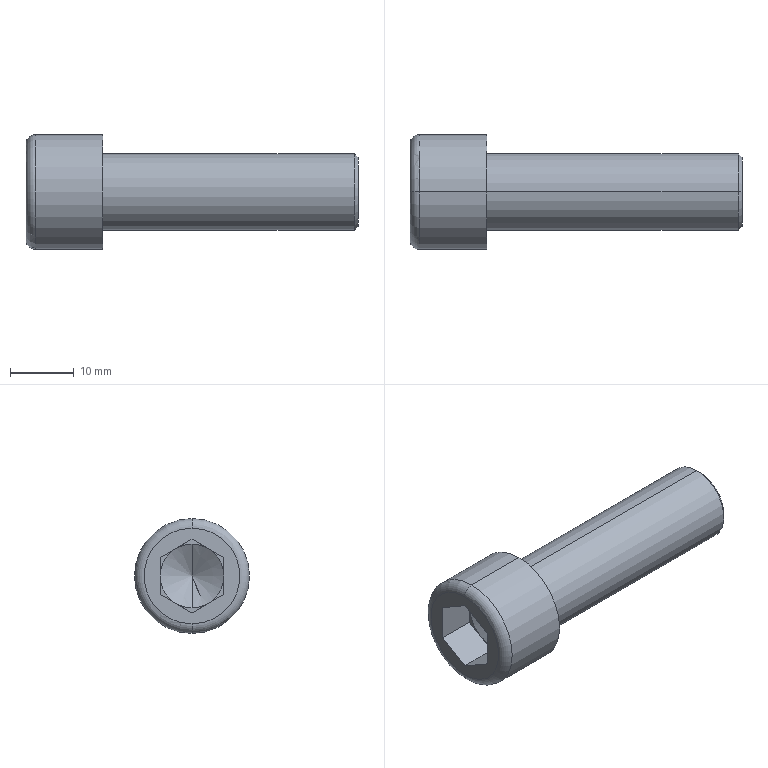Part | SolidWorks | features BaseBody 1 | 1 solid | 25 faces | box 52 x 18 x 18 mm | volume 6949 mm3 | plane 15 | cone 4 | cylinder 4 | torus 2 | commonest cylinder face diameters 12 x2 18 x2
STEP:
#1=CARTESIAN_POINT('',(52.,0.,-5.4));
#2=VERTEX_POINT('',#1);
#3=CARTESIAN_POINT('',(52.,0.,5.4));
#4=VERTEX_POINT('',#3);
#5=CARTESIAN_POINT('',(52.,0.,0.));
#6=DIRECTION('',(1.,0.,0.));
#7=DIRECTION('',(0.,0.,-1.));
#8=AXIS2_PLACEMENT_3D('',#5,#6,#7);
#9=CIRCLE('',#8,5.4);
#10=EDGE_CURVE('',#2,#4,#9,.T.);
#11=ORIENTED_EDGE('',*,*,#10,.F.);
#12=CARTESIAN_POINT('',(51.4,0.,-6.));
#13=VERTEX_POINT('',#12);
#14=CARTESIAN_POINT('',(52.,0.,-5.4));
#15=DIRECTION('',(-0.7071,0.,-0.7071));
#16=VECTOR('',#15,1000.);
#17=LINE('',#14,#16);
#18=EDGE_CURVE('',#2,#13,#17,.T.);
#19=ORIENTED_EDGE('',*,*,#18,.T.);
#20=CARTESIAN_POINT('',(51.4,0.,6.));
#21=VERTEX_POINT('',#20);
#22=CARTESIAN_POINT('',(51.4,0.,0.));
#23=DIRECTION('',(-1.,0.,0.));
#24=DIRECTION('',(0.,0.,-1.));
#25=AXIS2_PLACEMENT_3D('',#22,#23,#24);
#26=CIRCLE('',#25,6.);
#27=EDGE_CURVE('',#21,#13,#26,.T.);
#28=ORIENTED_EDGE('',*,*,#27,.F.);
#29=CARTESIAN_POINT('',(52.,0.,5.4));
#30=DIRECTION('',(-0.7071,0.,0.7071));
#31=VECTOR('',#30,1000.);
#32=LINE('',#29,#31);
#33=EDGE_CURVE('',#4,#21,#32,.T.);
#34=ORIENTED_EDGE('',*,*,#33,.F.);
#35=EDGE_LOOP('',(#11,#19,#28,#34));
#36=FACE_OUTER_BOUND('',#35,.T.);
#37=CARTESIAN_POINT('',(52.,0.,0.));
#38=DIRECTION('',(-1.,0.,0.));
#39=DIRECTION('',(0.,0.,1.));
#40=AXIS2_PLACEMENT_3D('',#37,#38,#39);
#41=CONICAL_SURFACE('',#40,5.4,0.7854);
#42=ADVANCED_FACE('',(#36),#41,.T.);
#43=CARTESIAN_POINT('',(0.,0.,7.5));
#44=VERTEX_POINT('',#43);
#45=CARTESIAN_POINT('',(0.,0.,-7.5));
#46=VERTEX_POINT('',#45);
#47=CARTESIAN_POINT('',(0.,0.,0.));
#48=DIRECTION('',(-1.,0.,0.));
#49=DIRECTION('',(0.,0.,-1.));
#50=AXIS2_PLACEMENT_3D('',#47,#48,#49);
#51=CIRCLE('',#50,7.5);
#52=EDGE_CURVE('',#44,#46,#51,.T.);
#53=ORIENTED_EDGE('',*,*,#52,.F.);
#54=CARTESIAN_POINT('',(1.5,0.,9.));
#55=VERTEX_POINT('',#54);
#56=CARTESIAN_POINT('',(1.5,0.,7.5));
#57=DIRECTION('',(0.,1.,0.));
#58=DIRECTION('',(0.,0.,1.));
#59=AXIS2_PLACEMENT_3D('',#56,#57,#58);
#60=CIRCLE('',#59,1.5);
#61=EDGE_CURVE('',#44,#55,#60,.T.);
#62=ORIENTED_EDGE('',*,*,#61,.T.);
#63=CARTESIAN_POINT('',(1.5,0.,-9.));
#64=VERTEX_POINT('',#63);
#65=CARTESIAN_POINT('',(1.5,0.,0.));
#66=DIRECTION('',(1.,0.,0.));
#67=DIRECTION('',(0.,0.,-1.));
#68=AXIS2_PLACEMENT_3D('',#65,#66,#67);
#69=CIRCLE('',#68,9.);
#70=EDGE_CURVE('',#64,#55,#69,.T.);
#71=ORIENTED_EDGE('',*,*,#70,.F.);
#72=CARTESIAN_POINT('',(1.5,0.,-7.5));
#73=DIRECTION('',(0.,-1.,0.));
#74=DIRECTION('',(0.,0.,-1.));
#75=AXIS2_PLACEMENT_3D('',#72,#73,#74);
#76=CIRCLE('',#75,1.5);
#77=EDGE_CURVE('',#46,#64,#76,.T.);
#78=ORIENTED_EDGE('',*,*,#77,.F.);
#79=EDGE_LOOP('',(#53,#62,#71,#78));
#80=FACE_OUTER_BOUND('',#79,.T.);
#81=CARTESIAN_POINT('',(1.5,0.,0.));
#82=DIRECTION('',(1.,0.,0.));
#83=DIRECTION('',(0.,0.,-1.));
#84=AXIS2_PLACEMENT_3D('',#81,#82,#83);
#85=TOROIDAL_SURFACE('',#84,7.5,1.5);
#86=ADVANCED_FACE('',(#80),#85,.T.);
#87=CARTESIAN_POINT('',(8.887,0.,0.));
#88=VERTEX_POINT('',#87);
#89=CARTESIAN_POINT('',(6.,0.,5.));
#90=VERTEX_POINT('',#89);
#91=CARTESIAN_POINT('',(6.,0.,5.));
#92=DIRECTION('',(-0.5,0.,0.866));
#93=VECTOR('',#92,1000.);
#94=LINE('',#91,#93);
#95=EDGE_CURVE('',#88,#90,#94,.T.);
#96=ORIENTED_EDGE('',*,*,#95,.F.);
#97=CARTESIAN_POINT('',(6.,0.,-5.));
#98=VERTEX_POINT('',#97);
#99=CARTESIAN_POINT('',(6.,0.,-5.));
#100=DIRECTION('',(-0.5,0.,-0.866));
#101=VECTOR('',#100,1000.);
#102=LINE('',#99,#101);
#103=EDGE_CURVE('',#88,#98,#102,.T.);
#104=ORIENTED_EDGE('',*,*,#103,.T.);
#105=CARTESIAN_POINT('',(6.,-2.5,-4.33));
#106=VERTEX_POINT('',#105);
#107=CARTESIAN_POINT('',(6.,0.,0.));
#108=DIRECTION('',(-1.,0.,0.));
#109=DIRECTION('',(0.,0.,-1.));
#110=AXIS2_PLACEMENT_3D('',#107,#108,#109);
#111=CIRCLE('',#110,5.);
#112=EDGE_CURVE('',#98,#106,#111,.T.);
#113=ORIENTED_EDGE('',*,*,#112,.T.);
#114=CARTESIAN_POINT('',(6.,-5.,0.));
#115=VERTEX_POINT('',#114);
#116=CARTESIAN_POINT('',(6.,0.,0.));
#117=DIRECTION('',(-1.,0.,0.));
#118=DIRECTION('',(0.,0.,-1.));
#119=AXIS2_PLACEMENT_3D('',#116,#117,#118);
#120=CIRCLE('',#119,5.);
#121=EDGE_CURVE('',#106,#115,#120,.T.);
#122=ORIENTED_EDGE('',*,*,#121,.T.);
#123=CARTESIAN_POINT('',(6.,-2.5,4.33));
#124=VERTEX_POINT('',#123);
#125=CARTESIAN_POINT('',(6.,0.,0.));
#126=DIRECTION('',(-1.,0.,0.));
#127=DIRECTION('',(0.,0.,-1.));
#128=AXIS2_PLACEMENT_3D('',#125,#126,#127);
#129=CIRCLE('',#128,5.);
#130=EDGE_CURVE('',#115,#124,#129,.T.);
#131=ORIENTED_EDGE('',*,*,#130,.T.);
#132=CARTESIAN_POINT('',(6.,0.,0.));
#133=DIRECTION('',(-1.,0.,0.));
#134=DIRECTION('',(0.,0.,-1.));
#135=AXIS2_PLACEMENT_3D('',#132,#133,#134);
#136=CIRCLE('',#135,5.);
#137=EDGE_CURVE('',#124,#90,#136,.T.);
#138=ORIENTED_EDGE('',*,*,#137,.T.);
#139=EDGE_LOOP('',(#96,#104,#113,#122,#131,#138));
#140=FACE_OUTER_BOUND('',#139,.T.);
#141=CARTESIAN_POINT('',(6.,0.,0.));
#142=DIRECTION('',(-1.,0.,0.));
#143=DIRECTION('',(0.,0.,1.));
#144=AXIS2_PLACEMENT_3D('',#141,#142,#143);
#145=CONICAL_SURFACE('',#144,5.,1.047);
#146=ADVANCED_FACE('',(#140),#145,.F.);
#147=ORIENTED_EDGE('',*,*,#27,.T.);
#148=CARTESIAN_POINT('',(12.,0.,-6.));
#149=VERTEX_POINT('',#148);
#150=CARTESIAN_POINT('',(52.,0.,-6.));
#151=DIRECTION('',(-1.,0.,0.));
#152=VECTOR('',#151,1000.);
#153=LINE('',#150,#152);
#154=EDGE_CURVE('',#13,#149,#153,.T.);
#155=ORIENTED_EDGE('',*,*,#154,.T.);
#156=CARTESIAN_POINT('',(12.,0.,6.));
#157=VERTEX_POINT('',#156);
#158=CARTESIAN_POINT('',(12.,0.,0.));
#159=DIRECTION('',(1.,0.,0.));
#160=DIRECTION('',(0.,0.,-1.));
#161=AXIS2_PLACEMENT_3D('',#158,#159,#160);
#162=CIRCLE('',#161,6.);
#163=EDGE_CURVE('',#149,#157,#162,.T.);
#164=ORIENTED_EDGE('',*,*,#163,.T.);
#165=CARTESIAN_POINT('',(52.,0.,6.));
#166=DIRECTION('',(-1.,0.,0.));
#167=VECTOR('',#166,1000.);
#168=LINE('',#165,#167);
#169=EDGE_CURVE('',#21,#157,#168,.T.);
#170=ORIENTED_EDGE('',*,*,#169,.F.);
#171=EDGE_LOOP('',(#147,#155,#164,#170));
#172=FACE_OUTER_BOUND('',#171,.T.);
#173=CARTESIAN_POINT('',(52.,0.,0.));
#174=DIRECTION('',(-1.,0.,0.));
#175=DIRECTION('',(0.,0.,1.));
#176=AXIS2_PLACEMENT_3D('',#173,#174,#175);
#177=CYLINDRICAL_SURFACE('',#176,6.);
#178=ADVANCED_FACE('',(#172),#177,.T.);
#179=CARTESIAN_POINT('',(12.,0.,-9.));
#180=VERTEX_POINT('',#179);
#181=CARTESIAN_POINT('',(12.,0.,9.));
#182=VERTEX_POINT('',#181);
#183=CARTESIAN_POINT('',(12.,0.,0.));
#184=DIRECTION('',(1.,0.,0.));
#185=DIRECTION('',(0.,0.,-1.));
#186=AXIS2_PLACEMENT_3D('',#183,#184,#185);
#187=CIRCLE('',#186,9.);
#188=EDGE_CURVE('',#180,#182,#187,.T.);
#189=ORIENTED_EDGE('',*,*,#188,.F.);
#190=CARTESIAN_POINT('',(12.,0.,-9.));
#191=DIRECTION('',(-1.,0.,0.));
#192=VECTOR('',#191,1000.);
#193=LINE('',#190,#192);
#194=EDGE_CURVE('',#180,#64,#193,.T.);
#195=ORIENTED_EDGE('',*,*,#194,.T.);
#196=ORIENTED_EDGE('',*,*,#70,.T.);
#197=CARTESIAN_POINT('',(12.,0.,9.));
#198=DIRECTION('',(-1.,0.,0.));
#199=VECTOR('',#198,1000.);
#200=LINE('',#197,#199);
#201=EDGE_CURVE('',#182,#55,#200,.T.);
#202=ORIENTED_EDGE('',*,*,#201,.F.);
#203=EDGE_LOOP('',(#189,#195,#196,#202));
#204=FACE_OUTER_BOUND('',#203,.T.);
#205=CARTESIAN_POINT('',(12.,0.,0.));
#206=DIRECTION('',(-1.,0.,0.));
#207=DIRECTION('',(0.,0.,1.));
#208=AXIS2_PLACEMENT_3D('',#205,#206,#207);
#209=CYLINDRICAL_SURFACE('',#208,9.);
#210=ADVANCED_FACE('',(#204),#209,.T.);
#211=CARTESIAN_POINT('',(0.,-5.,2.887));
#212=VERTEX_POINT('',#211);
#213=CARTESIAN_POINT('',(0.,-5.,-2.887));
#214=VERTEX_POINT('',#213);
#215=CARTESIAN_POINT('',(0.,-5.,2.887));
#216=DIRECTION('',(0.,0.,-1.));
#217=VECTOR('',#216,1000.);
#218=LINE('',#215,#217);
#219=EDGE_CURVE('',#212,#214,#218,.T.);
#220=ORIENTED_EDGE('',*,*,#219,.F.);
#221=CARTESIAN_POINT('',(6.,-5.,2.887));
#222=VERTEX_POINT('',#221);
#223=CARTESIAN_POINT('',(6.,-5.,2.887));
#224=DIRECTION('',(-1.,0.,0.));
#225=VECTOR('',#224,1000.);
#226=LINE('',#223,#225);
#227=EDGE_CURVE('',#222,#212,#226,.T.);
#228=ORIENTED_EDGE('',*,*,#227,.F.);
#229=CARTESIAN_POINT('',(6.,-5.,2.887));
#230=DIRECTION('',(0.,0.,-1.));
#231=VECTOR('',#230,1000.);
#232=LINE('',#229,#231);
#233=EDGE_CURVE('',#222,#115,#232,.T.);
#234=ORIENTED_EDGE('',*,*,#233,.T.);
#235=CARTESIAN_POINT('',(6.,-5.,-2.887));
#236=VERTEX_POINT('',#235);
#237=CARTESIAN_POINT('',(6.,-5.,2.887));
#238=DIRECTION('',(0.,0.,-1.));
#239=VECTOR('',#238,1000.);
#240=LINE('',#237,#239);
#241=EDGE_CURVE('',#115,#236,#240,.T.);
#242=ORIENTED_EDGE('',*,*,#241,.T.);
#243=CARTESIAN_POINT('',(6.,-5.,-2.887));
#244=DIRECTION('',(-1.,0.,0.));
#245=VECTOR('',#244,1000.);
#246=LINE('',#243,#245);
#247=EDGE_CURVE('',#236,#214,#246,.T.);
#248=ORIENTED_EDGE('',*,*,#247,.T.);
#249=EDGE_LOOP('',(#220,#228,#234,#242,#248));
#250=FACE_OUTER_BOUND('',#249,.T.);
#251=CARTESIAN_POINT('',(6.,-5.,2.887));
#252=DIRECTION('',(0.,1.,0.));
#253=DIRECTION('',(1.,0.,0.));
#254=AXIS2_PLACEMENT_3D('',#251,#252,#253);
#255=PLANE('',#254);
#256=ADVANCED_FACE('',(#250),#255,.T.);
#257=CARTESIAN_POINT('',(0.,0.,5.774));
#258=VERTEX_POINT('',#257);
#259=CARTESIAN_POINT('',(0.,0.,5.774));
#260=DIRECTION('',(0.,-0.866,-0.5));
#261=VECTOR('',#260,1000.);
#262=LINE('',#259,#261);
#263=EDGE_CURVE('',#258,#212,#262,.T.);
#264=ORIENTED_EDGE('',*,*,#263,.F.);
#265=CARTESIAN_POINT('',(6.,0.,5.774));
#266=VERTEX_POINT('',#265);
#267=CARTESIAN_POINT('',(6.,0.,5.774));
#268=DIRECTION('',(-1.,0.,0.));
#269=VECTOR('',#268,1000.);
#270=LINE('',#267,#269);
#271=EDGE_CURVE('',#266,#258,#270,.T.);
#272=ORIENTED_EDGE('',*,*,#271,.F.);
#273=CARTESIAN_POINT('',(6.,0.,5.774));
#274=DIRECTION('',(0.,-0.866,-0.5));
#275=VECTOR('',#274,1000.);
#276=LINE('',#273,#275);
#277=EDGE_CURVE('',#266,#124,#276,.T.);
#278=ORIENTED_EDGE('',*,*,#277,.T.);
#279=CARTESIAN_POINT('',(6.,0.,5.774));
#280=DIRECTION('',(0.,-0.866,-0.5));
#281=VECTOR('',#280,1000.);
#282=LINE('',#279,#281);
#283=EDGE_CURVE('',#124,#222,#282,.T.);
#284=ORIENTED_EDGE('',*,*,#283,.T.);
#285=ORIENTED_EDGE('',*,*,#227,.T.);
#286=EDGE_LOOP('',(#264,#272,#278,#284,#285));
#287=FACE_OUTER_BOUND('',#286,.T.);
#288=CARTESIAN_POINT('',(6.,0.,5.774));
#289=DIRECTION('',(0.,0.5,-0.866));
#290=DIRECTION('',(-1.,0.,0.));
#291=AXIS2_PLACEMENT_3D('',#288,#289,#290);
#292=PLANE('',#291);
#293=ADVANCED_FACE('',(#287),#292,.T.);
#294=CARTESIAN_POINT('',(0.,5.,2.887));
#295=VERTEX_POINT('',#294);
#296=CARTESIAN_POINT('',(0.,5.,2.887));
#297=DIRECTION('',(0.,-0.866,0.5));
#298=VECTOR('',#297,1000.);
#299=LINE('',#296,#298);
#300=EDGE_CURVE('',#295,#258,#299,.T.);
#301=ORIENTED_EDGE('',*,*,#300,.F.);
#302=CARTESIAN_POINT('',(6.,5.,2.887));
#303=VERTEX_POINT('',#302);
#304=CARTESIAN_POINT('',(6.,5.,2.887));
#305=DIRECTION('',(-1.,0.,0.));
#306=VECTOR('',#305,1000.);
#307=LINE('',#304,#306);
#308=EDGE_CURVE('',#303,#295,#307,.T.);
#309=ORIENTED_EDGE('',*,*,#308,.F.);
#310=CARTESIAN_POINT('',(6.,2.5,4.33));
#311=VERTEX_POINT('',#310);
#312=CARTESIAN_POINT('',(6.,5.,2.887));
#313=DIRECTION('',(0.,-0.866,0.5));
#314=VECTOR('',#313,1000.);
#315=LINE('',#312,#314);
#316=EDGE_CURVE('',#303,#311,#315,.T.);
#317=ORIENTED_EDGE('',*,*,#316,.T.);
#318=CARTESIAN_POINT('',(6.,5.,2.887));
#319=DIRECTION('',(0.,-0.866,0.5));
#320=VECTOR('',#319,1000.);
#321=LINE('',#318,#320);
#322=EDGE_CURVE('',#311,#266,#321,.T.);
#323=ORIENTED_EDGE('',*,*,#322,.T.);
#324=ORIENTED_EDGE('',*,*,#271,.T.);
#325=EDGE_LOOP('',(#301,#309,#317,#323,#324));
#326=FACE_OUTER_BOUND('',#325,.T.);
#327=CARTESIAN_POINT('',(6.,5.,2.887));
#328=DIRECTION('',(0.,-0.5,-0.866));
#329=DIRECTION('',(0.,-0.866,0.5));
#330=AXIS2_PLACEMENT_3D('',#327,#328,#329);
#331=PLANE('',#330);
#332=ADVANCED_FACE('',(#326),#331,.T.);
#333=CARTESIAN_POINT('',(0.,5.,-2.887));
#334=VERTEX_POINT('',#333);
#335=CARTESIAN_POINT('',(0.,5.,-2.887));
#336=DIRECTION('',(0.,0.,1.));
#337=VECTOR('',#336,1000.);
#338=LINE('',#335,#337);
#339=EDGE_CURVE('',#334,#295,#338,.T.);
#340=ORIENTED_EDGE('',*,*,#339,.F.);
#341=CARTESIAN_POINT('',(6.,5.,-2.887));
#342=VERTEX_POINT('',#341);
#343=CARTESIAN_POINT('',(6.,5.,-2.887));
#344=DIRECTION('',(-1.,0.,0.));
#345=VECTOR('',#344,1000.);
#346=LINE('',#343,#345);
#347=EDGE_CURVE('',#342,#334,#346,.T.);
#348=ORIENTED_EDGE('',*,*,#347,.F.);
#349=CARTESIAN_POINT('',(6.,5.,0.));
#350=VERTEX_POINT('',#349);
#351=CARTESIAN_POINT('',(6.,5.,-2.887));
#352=DIRECTION('',(0.,0.,1.));
#353=VECTOR('',#352,1000.);
#354=LINE('',#351,#353);
#355=EDGE_CURVE('',#342,#350,#354,.T.);
#356=ORIENTED_EDGE('',*,*,#355,.T.);
#357=CARTESIAN_POINT('',(6.,5.,-2.887));
#358=DIRECTION('',(0.,0.,1.));
#359=VECTOR('',#358,1000.);
#360=LINE('',#357,#359);
#361=EDGE_CURVE('',#350,#303,#360,.T.);
#362=ORIENTED_EDGE('',*,*,#361,.T.);
#363=ORIENTED_EDGE('',*,*,#308,.T.);
#364=EDGE_LOOP('',(#340,#348,#356,#362,#363));
#365=FACE_OUTER_BOUND('',#364,.T.);
#366=CARTESIAN_POINT('',(6.,5.,-2.887));
#367=DIRECTION('',(0.,-1.,0.));
#368=DIRECTION('',(0.,0.,-1.));
#369=AXIS2_PLACEMENT_3D('',#366,#367,#368);
#370=PLANE('',#369);
#371=ADVANCED_FACE('',(#365),#370,.T.);
#372=CARTESIAN_POINT('',(0.,0.,-5.774));
#373=VERTEX_POINT('',#372);
#374=CARTESIAN_POINT('',(0.,0.,-5.774));
#375=DIRECTION('',(0.,0.866,0.5));
#376=VECTOR('',#375,1000.);
#377=LINE('',#374,#376);
#378=EDGE_CURVE('',#373,#334,#377,.T.);
#379=ORIENTED_EDGE('',*,*,#378,.F.);
#380=CARTESIAN_POINT('',(6.,0.,-5.774));
#381=VERTEX_POINT('',#380);
#382=CARTESIAN_POINT('',(6.,0.,-5.774));
#383=DIRECTION('',(-1.,0.,0.));
#384=VECTOR('',#383,1000.);
#385=LINE('',#382,#384);
#386=EDGE_CURVE('',#381,#373,#385,.T.);
#387=ORIENTED_EDGE('',*,*,#386,.F.);
#388=CARTESIAN_POINT('',(6.,2.5,-4.33));
#389=VERTEX_POINT('',#388);
#390=CARTESIAN_POINT('',(6.,0.,-5.774));
#391=DIRECTION('',(0.,0.866,0.5));
#392=VECTOR('',#391,1000.);
#393=LINE('',#390,#392);
#394=EDGE_CURVE('',#381,#389,#393,.T.);
#395=ORIENTED_EDGE('',*,*,#394,.T.);
#396=CARTESIAN_POINT('',(6.,0.,-5.774));
#397=DIRECTION('',(0.,0.866,0.5));
#398=VECTOR('',#397,1000.);
#399=LINE('',#396,#398);
#400=EDGE_CURVE('',#389,#342,#399,.T.);
#401=ORIENTED_EDGE('',*,*,#400,.T.);
#402=ORIENTED_EDGE('',*,*,#347,.T.);
#403=EDGE_LOOP('',(#379,#387,#395,#401,#402));
#404=FACE_OUTER_BOUND('',#403,.T.);
#405=CARTESIAN_POINT('',(6.,0.,-5.774));
#406=DIRECTION('',(0.,-0.5,0.866));
#407=DIRECTION('',(-1.,0.,0.));
#408=AXIS2_PLACEMENT_3D('',#405,#406,#407);
#409=PLANE('',#408);
#410=ADVANCED_FACE('',(#404),#409,.T.);
#411=CARTESIAN_POINT('',(0.,-5.,-2.887));
#412=DIRECTION('',(0.,0.866,-0.5));
#413=VECTOR('',#412,1000.);
#414=LINE('',#411,#413);
#415=EDGE_CURVE('',#214,#373,#414,.T.);
#416=ORIENTED_EDGE('',*,*,#415,.F.);
#417=ORIENTED_EDGE('',*,*,#247,.F.);
#418=CARTESIAN_POINT('',(6.,-5.,-2.887));
#419=DIRECTION('',(0.,0.866,-0.5));
#420=VECTOR('',#419,1000.);
#421=LINE('',#418,#420);
#422=EDGE_CURVE('',#236,#106,#421,.T.);
#423=ORIENTED_EDGE('',*,*,#422,.T.);
#424=CARTESIAN_POINT('',(6.,-5.,-2.887));
#425=DIRECTION('',(0.,0.866,-0.5));
#426=VECTOR('',#425,1000.);
#427=LINE('',#424,#426);
#428=EDGE_CURVE('',#106,#381,#427,.T.);
#429=ORIENTED_EDGE('',*,*,#428,.T.);
#430=ORIENTED_EDGE('',*,*,#386,.T.);
#431=EDGE_LOOP('',(#416,#417,#423,#429,#430));
#432=FACE_OUTER_BOUND('',#431,.T.);
#433=CARTESIAN_POINT('',(6.,-5.,-2.887));
#434=DIRECTION('',(0.,0.5,0.866));
#435=DIRECTION('',(1.,0.,0.));
#436=AXIS2_PLACEMENT_3D('',#433,#434,#435);
#437=PLANE('',#436);
#438=ADVANCED_FACE('',(#432),#437,.T.);
#439=CARTESIAN_POINT('',(52.,0.,0.));
#440=DIRECTION('',(1.,0.,0.));
#441=DIRECTION('',(0.,0.,-1.));
#442=AXIS2_PLACEMENT_3D('',#439,#440,#441);
#443=CIRCLE('',#442,5.4);
#444=EDGE_CURVE('',#4,#2,#443,.T.);
#445=ORIENTED_EDGE('',*,*,#444,.T.);
#446=ORIENTED_EDGE('',*,*,#10,.T.);
#447=EDGE_LOOP('',(#445,#446));
#448=FACE_OUTER_BOUND('',#447,.T.);
#449=CARTESIAN_POINT('',(52.,0.,0.));
#450=DIRECTION('',(1.,0.,0.));
#451=DIRECTION('',(0.,1.,0.));
#452=AXIS2_PLACEMENT_3D('',#449,#450,#451);
#453=PLANE('',#452);
#454=ADVANCED_FACE('',(#448),#453,.T.);
#455=CARTESIAN_POINT('',(12.,0.,0.));
#456=DIRECTION('',(1.,0.,0.));
#457=DIRECTION('',(0.,0.,-1.));
#458=AXIS2_PLACEMENT_3D('',#455,#456,#457);
#459=CIRCLE('',#458,6.);
#460=EDGE_CURVE('',#157,#149,#459,.T.);
#461=ORIENTED_EDGE('',*,*,#460,.F.);
#462=ORIENTED_EDGE('',*,*,#163,.F.);
#463=EDGE_LOOP('',(#461,#462));
#464=FACE_BOUND('',#463,.T.);
#465=CARTESIAN_POINT('',(12.,0.,0.));
#466=DIRECTION('',(1.,0.,0.));
#467=DIRECTION('',(0.,0.,-1.));
#468=AXIS2_PLACEMENT_3D('',#465,#466,#467);
#469=CIRCLE('',#468,9.);
#470=EDGE_CURVE('',#182,#180,#469,.T.);
#471=ORIENTED_EDGE('',*,*,#470,.T.);
#472=ORIENTED_EDGE('',*,*,#188,.T.);
#473=EDGE_LOOP('',(#471,#472));
#474=FACE_OUTER_BOUND('',#473,.T.);
#475=CARTESIAN_POINT('',(12.,0.,0.));
#476=DIRECTION('',(1.,0.,0.));
#477=DIRECTION('',(0.,1.,0.));
#478=AXIS2_PLACEMENT_3D('',#475,#476,#477);
#479=PLANE('',#478);
#480=ADVANCED_FACE('',(#464,#474),#479,.T.);
#481=ORIENTED_EDGE('',*,*,#415,.T.);
#482=ORIENTED_EDGE('',*,*,#378,.T.);
#483=ORIENTED_EDGE('',*,*,#339,.T.);
#484=ORIENTED_EDGE('',*,*,#300,.T.);
#485=ORIENTED_EDGE('',*,*,#263,.T.);
#486=ORIENTED_EDGE('',*,*,#219,.T.);
#487=EDGE_LOOP('',(#481,#482,#483,#484,#485,#486));
#488=FACE_BOUND('',#487,.T.);
#489=CARTESIAN_POINT('',(0.,0.,0.));
#490=DIRECTION('',(-1.,0.,0.));
#491=DIRECTION('',(0.,0.,-1.));
#492=AXIS2_PLACEMENT_3D('',#489,#490,#491);
#493=CIRCLE('',#492,7.5);
#494=EDGE_CURVE('',#46,#44,#493,.T.);
#495=ORIENTED_EDGE('',*,*,#494,.T.);
#496=ORIENTED_EDGE('',*,*,#52,.T.);
#497=EDGE_LOOP('',(#495,#496));
#498=FACE_OUTER_BOUND('',#497,.T.);
#499=CARTESIAN_POINT('',(0.,0.,0.));
#500=DIRECTION('',(1.,0.,0.));
#501=DIRECTION('',(0.,1.,0.));
#502=AXIS2_PLACEMENT_3D('',#499,#500,#501);
#503=PLANE('',#502);
#504=ADVANCED_FACE('',(#488,#498),#503,.F.);
#505=CARTESIAN_POINT('',(6.,0.,0.));
#506=DIRECTION('',(-1.,0.,0.));
#507=DIRECTION('',(0.,0.,-1.));
#508=AXIS2_PLACEMENT_3D('',#505,#506,#507);
#509=CIRCLE('',#508,5.);
#510=EDGE_CURVE('',#389,#98,#509,.T.);
#511=ORIENTED_EDGE('',*,*,#510,.F.);
#512=ORIENTED_EDGE('',*,*,#394,.F.);
#513=ORIENTED_EDGE('',*,*,#428,.F.);
#514=ORIENTED_EDGE('',*,*,#112,.F.);
#515=EDGE_LOOP('',(#511,#512,#513,#514));
#516=FACE_OUTER_BOUND('',#515,.T.);
#517=CARTESIAN_POINT('',(6.,0.,-5.774));
#518=DIRECTION('',(1.,0.,0.));
#519=DIRECTION('',(0.,1.,0.));
#520=AXIS2_PLACEMENT_3D('',#517,#518,#519);
#521=PLANE('',#520);
#522=ADVANCED_FACE('',(#516),#521,.F.);
#523=CARTESIAN_POINT('',(6.,0.,0.));
#524=DIRECTION('',(1.,0.,0.));
#525=DIRECTION('',(0.,0.,-1.));
#526=AXIS2_PLACEMENT_3D('',#523,#524,#525);
#527=CIRCLE('',#526,5.);
#528=EDGE_CURVE('',#389,#350,#527,.T.);
#529=ORIENTED_EDGE('',*,*,#528,.T.);
#530=ORIENTED_EDGE('',*,*,#355,.F.);
#531=ORIENTED_EDGE('',*,*,#400,.F.);
#532=EDGE_LOOP('',(#529,#530,#531));
#533=FACE_OUTER_BOUND('',#532,.T.);
#534=CARTESIAN_POINT('',(6.,0.,-5.774));
#535=DIRECTION('',(1.,0.,0.));
#536=DIRECTION('',(0.,1.,0.));
#537=AXIS2_PLACEMENT_3D('',#534,#535,#536);
#538=PLANE('',#537);
#539=ADVANCED_FACE('',(#533),#538,.F.);
#540=CARTESIAN_POINT('',(6.,0.,0.));
#541=DIRECTION('',(-1.,0.,0.));
#542=DIRECTION('',(0.,0.,-1.));
#543=AXIS2_PLACEMENT_3D('',#540,#541,#542);
#544=CIRCLE('',#543,5.);
#545=EDGE_CURVE('',#311,#350,#544,.T.);
#546=ORIENTED_EDGE('',*,*,#545,.F.);
#547=ORIENTED_EDGE('',*,*,#316,.F.);
#548=ORIENTED_EDGE('',*,*,#361,.F.);
#549=EDGE_LOOP('',(#546,#547,#548));
#550=FACE_OUTER_BOUND('',#549,.T.);
#551=CARTESIAN_POINT('',(6.,0.,-5.774));
#552=DIRECTION('',(1.,0.,0.));
#553=DIRECTION('',(0.,1.,0.));
#554=AXIS2_PLACEMENT_3D('',#551,#552,#553);
#555=PLANE('',#554);
#556=ADVANCED_FACE('',(#550),#555,.F.);
#557=ORIENTED_EDGE('',*,*,#137,.F.);
#558=ORIENTED_EDGE('',*,*,#277,.F.);
#559=ORIENTED_EDGE('',*,*,#322,.F.);
#560=CARTESIAN_POINT('',(6.,0.,0.));
#561=DIRECTION('',(-1.,0.,0.));
#562=DIRECTION('',(0.,0.,-1.));
#563=AXIS2_PLACEMENT_3D('',#560,#561,#562);
#564=CIRCLE('',#563,5.);
#565=EDGE_CURVE('',#90,#311,#564,.T.);
#566=ORIENTED_EDGE('',*,*,#565,.F.);
#567=EDGE_LOOP('',(#557,#558,#559,#566));
#568=FACE_OUTER_BOUND('',#567,.T.);
#569=CARTESIAN_POINT('',(6.,0.,-5.774));
#570=DIRECTION('',(1.,0.,0.));
#571=DIRECTION('',(0.,1.,0.));
#572=AXIS2_PLACEMENT_3D('',#569,#570,#571);
#573=PLANE('',#572);
#574=ADVANCED_FACE('',(#568),#573,.F.);
#575=ORIENTED_EDGE('',*,*,#130,.F.);
#576=ORIENTED_EDGE('',*,*,#233,.F.);
#577=ORIENTED_EDGE('',*,*,#283,.F.);
#578=EDGE_LOOP('',(#575,#576,#577));
#579=FACE_OUTER_BOUND('',#578,.T.);
#580=CARTESIAN_POINT('',(6.,0.,-5.774));
#581=DIRECTION('',(1.,0.,0.));
#582=DIRECTION('',(0.,1.,0.));
#583=AXIS2_PLACEMENT_3D('',#580,#581,#582);
#584=PLANE('',#583);
#585=ADVANCED_FACE('',(#579),#584,.F.);
#586=ORIENTED_EDGE('',*,*,#121,.F.);
#587=ORIENTED_EDGE('',*,*,#422,.F.);
#588=ORIENTED_EDGE('',*,*,#241,.F.);
#589=EDGE_LOOP('',(#586,#587,#588));
#590=FACE_OUTER_BOUND('',#589,.T.);
#591=CARTESIAN_POINT('',(6.,0.,-5.774));
#592=DIRECTION('',(1.,0.,0.));
#593=DIRECTION('',(0.,1.,0.));
#594=AXIS2_PLACEMENT_3D('',#591,#592,#593);
#595=PLANE('',#594);
#596=ADVANCED_FACE('',(#590),#595,.F.);
#597=ORIENTED_EDGE('',*,*,#194,.F.);
#598=ORIENTED_EDGE('',*,*,#470,.F.);
#599=ORIENTED_EDGE('',*,*,#201,.T.);
#600=CARTESIAN_POINT('',(1.5,0.,0.));
#601=DIRECTION('',(1.,0.,0.));
#602=DIRECTION('',(0.,0.,-1.));
#603=AXIS2_PLACEMENT_3D('',#600,#601,#602);
#604=CIRCLE('',#603,9.);
#605=EDGE_CURVE('',#55,#64,#604,.T.);
#606=ORIENTED_EDGE('',*,*,#605,.T.);
#607=EDGE_LOOP('',(#597,#598,#599,#606));
#608=FACE_OUTER_BOUND('',#607,.T.);
#609=CARTESIAN_POINT('',(12.,0.,0.));
#610=DIRECTION('',(-1.,0.,0.));
#611=DIRECTION('',(0.,0.,1.));
#612=AXIS2_PLACEMENT_3D('',#609,#610,#611);
#613=CYLINDRICAL_SURFACE('',#612,9.);
#614=ADVANCED_FACE('',(#608),#613,.T.);
#615=ORIENTED_EDGE('',*,*,#154,.F.);
#616=CARTESIAN_POINT('',(51.4,0.,0.));
#617=DIRECTION('',(-1.,0.,0.));
#618=DIRECTION('',(0.,0.,-1.));
#619=AXIS2_PLACEMENT_3D('',#616,#617,#618);
#620=CIRCLE('',#619,6.);
#621=EDGE_CURVE('',#13,#21,#620,.T.);
#622=ORIENTED_EDGE('',*,*,#621,.T.);
#623=ORIENTED_EDGE('',*,*,#169,.T.);
#624=ORIENTED_EDGE('',*,*,#460,.T.);
#625=EDGE_LOOP('',(#615,#622,#623,#624));
#626=FACE_OUTER_BOUND('',#625,.T.);
#627=CARTESIAN_POINT('',(52.,0.,0.));
#628=DIRECTION('',(-1.,0.,0.));
#629=DIRECTION('',(0.,0.,1.));
#630=AXIS2_PLACEMENT_3D('',#627,#628,#629);
#631=CYLINDRICAL_SURFACE('',#630,6.);
#632=ADVANCED_FACE('',(#626),#631,.T.);
#633=ORIENTED_EDGE('',*,*,#103,.F.);
#634=ORIENTED_EDGE('',*,*,#95,.T.);
#635=ORIENTED_EDGE('',*,*,#565,.T.);
#636=ORIENTED_EDGE('',*,*,#545,.T.);
#637=ORIENTED_EDGE('',*,*,#528,.F.);
#638=ORIENTED_EDGE('',*,*,#510,.T.);
#639=EDGE_LOOP('',(#633,#634,#635,#636,#637,#638));
#640=FACE_OUTER_BOUND('',#639,.T.);
#641=CARTESIAN_POINT('',(6.,0.,0.));
#642=DIRECTION('',(-1.,0.,0.));
#643=DIRECTION('',(0.,0.,1.));
#644=AXIS2_PLACEMENT_3D('',#641,#642,#643);
#645=CONICAL_SURFACE('',#644,5.,1.047);
#646=ADVANCED_FACE('',(#640),#645,.F.);
#647=ORIENTED_EDGE('',*,*,#61,.F.);
#648=ORIENTED_EDGE('',*,*,#494,.F.);
#649=ORIENTED_EDGE('',*,*,#77,.T.);
#650=ORIENTED_EDGE('',*,*,#605,.F.);
#651=EDGE_LOOP('',(#647,#648,#649,#650));
#652=FACE_OUTER_BOUND('',#651,.T.);
#653=CARTESIAN_POINT('',(1.5,0.,0.));
#654=DIRECTION('',(1.,0.,0.));
#655=DIRECTION('',(0.,0.,-1.));
#656=AXIS2_PLACEMENT_3D('',#653,#654,#655);
#657=TOROIDAL_SURFACE('',#656,7.5,1.5);
#658=ADVANCED_FACE('',(#652),#657,.T.);
#659=ORIENTED_EDGE('',*,*,#18,.F.);
#660=ORIENTED_EDGE('',*,*,#444,.F.);
#661=ORIENTED_EDGE('',*,*,#33,.T.);
#662=ORIENTED_EDGE('',*,*,#621,.F.);
#663=EDGE_LOOP('',(#659,#660,#661,#662));
#664=FACE_OUTER_BOUND('',#663,.T.);
#665=CARTESIAN_POINT('',(52.,0.,0.));
#666=DIRECTION('',(-1.,0.,0.));
#667=DIRECTION('',(0.,0.,1.));
#668=AXIS2_PLACEMENT_3D('',#665,#666,#667);
#669=CONICAL_SURFACE('',#668,5.4,0.7854);
#670=ADVANCED_FACE('',(#664),#669,.T.);
#671=CLOSED_SHELL('',(#42,#86,#146,#178,#210,#256,#293,#332,#371,#410,#438,#454,#480,#504,#522,#539,#556,#574,#585,#596,#614,#632,#646,#658,#670));
#672=MANIFOLD_SOLID_BREP('',#671);
#673=CARTESIAN_POINT('',(0.,0.,0.));
#674=DIRECTION('',(0.,0.,1.));
#675=DIRECTION('',(1.,0.,0.));
#676=AXIS2_PLACEMENT_3D('',#673,#674,#675);
#677=(LENGTH_UNIT()NAMED_UNIT(*)SI_UNIT(.MILLI.,.METRE.));
#678=UNCERTAINTY_MEASURE_WITH_UNIT(LENGTH_MEASURE(0.00001),#677,'','');
#679=(NAMED_UNIT(*)PLANE_ANGLE_UNIT()SI_UNIT($,.RADIAN.));
#680=(NAMED_UNIT(*)SI_UNIT($,.STERADIAN.)SOLID_ANGLE_UNIT());
#681=(GEOMETRIC_REPRESENTATION_CONTEXT(3)GLOBAL_UNCERTAINTY_ASSIGNED_CONTEXT((#678))GLOBAL_UNIT_ASSIGNED_CONTEXT((#677,#679,#680))REPRESENTATION_CONTEXT('',''));
#682=ADVANCED_BREP_SHAPE_REPRESENTATION('',(#672,#676),#681);